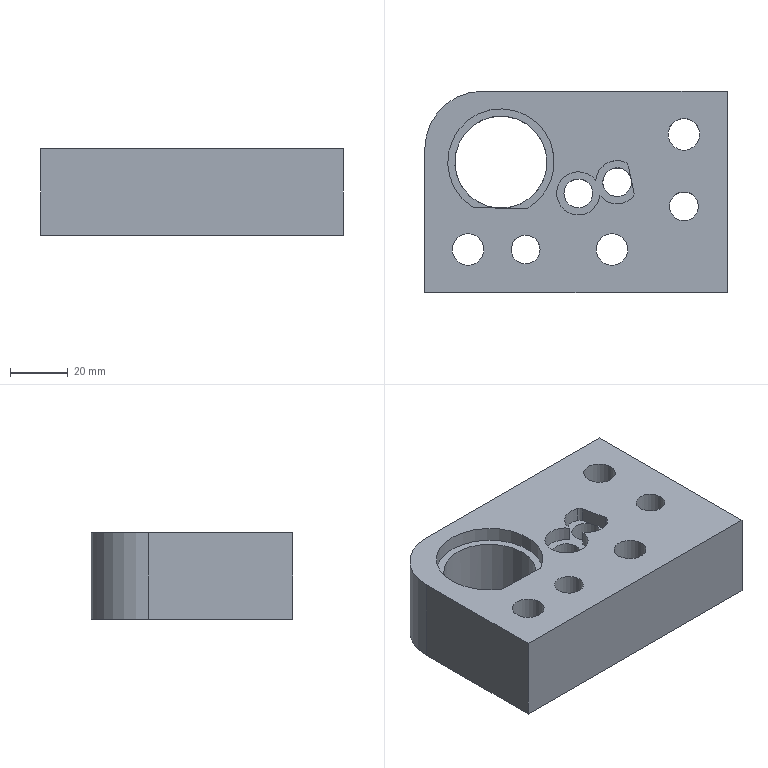Part | NX | features solid 2 | 1 solid | 33 faces | box 105 x 70 x 30 mm | volume 169797 mm3 | cylinder 20 | plane 13 | commonest cylinder face diameters 4 x4 10 x4 11 x3 15 x3 17 x3 32 x1
STEP:
#1=CARTESIAN_POINT('',(-270.,215.,109.));
#2=VERTEX_POINT('',#1);
#3=CARTESIAN_POINT('',(-275.,215.,109.));
#4=DIRECTION('',(0.,0.,1.));
#5=DIRECTION('',(1.,0.,0.));
#6=AXIS2_PLACEMENT_3D('',#3,#4,#5);
#7=CIRCLE('',#6,5.);
#8=EDGE_CURVE('',#2,#2,#7,.T.);
#9=ORIENTED_EDGE('',*,*,#8,.F.);
#10=EDGE_LOOP('',(#9));
#11=FACE_BOUND('',#10,.T.);
#12=CARTESIAN_POINT('',(-215.,230.,109.));
#13=VERTEX_POINT('',#12);
#14=CARTESIAN_POINT('',(-220.,230.,109.));
#15=DIRECTION('',(0.,0.,1.));
#16=DIRECTION('',(1.,0.,0.));
#17=AXIS2_PLACEMENT_3D('',#14,#15,#16);
#18=CIRCLE('',#17,5.);
#19=EDGE_CURVE('',#13,#13,#18,.T.);
#20=ORIENTED_EDGE('',*,*,#19,.F.);
#21=EDGE_LOOP('',(#20));
#22=FACE_BOUND('',#21,.T.);
#23=CARTESIAN_POINT('',(-289.5,215.,109.));
#24=VERTEX_POINT('',#23);
#25=CARTESIAN_POINT('',(-295.,215.,109.));
#26=DIRECTION('',(0.,0.,1.));
#27=DIRECTION('',(1.,0.,0.));
#28=AXIS2_PLACEMENT_3D('',#25,#26,#27);
#29=CIRCLE('',#28,5.5);
#30=EDGE_CURVE('',#24,#24,#29,.T.);
#31=ORIENTED_EDGE('',*,*,#30,.F.);
#32=EDGE_LOOP('',(#31));
#33=FACE_BOUND('',#32,.T.);
#34=CARTESIAN_POINT('',(-239.5,215.,109.));
#35=VERTEX_POINT('',#34);
#36=CARTESIAN_POINT('',(-245.,215.,109.));
#37=DIRECTION('',(0.,0.,1.));
#38=DIRECTION('',(1.,0.,0.));
#39=AXIS2_PLACEMENT_3D('',#36,#37,#38);
#40=CIRCLE('',#39,5.5);
#41=EDGE_CURVE('',#35,#35,#40,.T.);
#42=ORIENTED_EDGE('',*,*,#41,.F.);
#43=EDGE_LOOP('',(#42));
#44=FACE_BOUND('',#43,.T.);
#45=CARTESIAN_POINT('',(-214.5,255.,109.));
#46=VERTEX_POINT('',#45);
#47=CARTESIAN_POINT('',(-220.,255.,109.));
#48=DIRECTION('',(0.,0.,1.));
#49=DIRECTION('',(1.,0.,0.));
#50=AXIS2_PLACEMENT_3D('',#47,#48,#49);
#51=CIRCLE('',#50,5.5);
#52=EDGE_CURVE('',#46,#46,#51,.T.);
#53=ORIENTED_EDGE('',*,*,#52,.F.);
#54=EDGE_LOOP('',(#53));
#55=FACE_BOUND('',#54,.T.);
#56=CARTESIAN_POINT('',(-292.747,229.61,109.));
#57=VERTEX_POINT('',#56);
#58=CARTESIAN_POINT('',(-275.289,229.126,109.));
#59=VERTEX_POINT('',#58);
#60=CARTESIAN_POINT('',(-201.051,227.07,109.));
#61=DIRECTION('',(0.9996,-0.0277,0.));
#62=VECTOR('',#61,1000.);
#63=LINE('',#60,#62);
#64=EDGE_CURVE('',#57,#59,#63,.T.);
#65=ORIENTED_EDGE('',*,*,#64,.F.);
#66=CARTESIAN_POINT('',(-293.797,229.942,109.));
#67=VERTEX_POINT('',#66);
#68=CARTESIAN_POINT('',(-292.692,231.609,109.));
#69=DIRECTION('',(0.,0.,1.));
#70=DIRECTION('',(1.,0.,0.));
#71=AXIS2_PLACEMENT_3D('',#68,#69,#70);
#72=CIRCLE('',#71,2.);
#73=EDGE_CURVE('',#57,#67,#72,.F.);
#74=ORIENTED_EDGE('',*,*,#73,.T.);
#75=CARTESIAN_POINT('',(-274.223,229.4,109.));
#76=VERTEX_POINT('',#75);
#77=CARTESIAN_POINT('',(-283.575,245.362,109.));
#78=DIRECTION('',(0.,0.,1.));
#79=DIRECTION('',(1.,0.,0.));
#80=AXIS2_PLACEMENT_3D('',#77,#78,#79);
#81=CIRCLE('',#80,18.5);
#82=EDGE_CURVE('',#67,#76,#81,.F.);
#83=ORIENTED_EDGE('',*,*,#82,.T.);
#84=CARTESIAN_POINT('',(-275.234,231.126,109.));
#85=DIRECTION('',(0.,0.,1.));
#86=DIRECTION('',(1.,0.,0.));
#87=AXIS2_PLACEMENT_3D('',#84,#85,#86);
#88=CIRCLE('',#87,2.);
#89=EDGE_CURVE('',#76,#59,#88,.F.);
#90=ORIENTED_EDGE('',*,*,#89,.T.);
#91=EDGE_LOOP('',(#65,#74,#83,#90));
#92=FACE_BOUND('',#91,.T.);
#93=CARTESIAN_POINT('',(-290.,270.,109.));
#94=VERTEX_POINT('',#93);
#95=CARTESIAN_POINT('',(-205.,270.,109.));
#96=VERTEX_POINT('',#95);
#97=CARTESIAN_POINT('',(-310.,270.,109.));
#98=DIRECTION('',(1.,0.,0.));
#99=VECTOR('',#98,1000.);
#100=LINE('',#97,#99);
#101=EDGE_CURVE('',#94,#96,#100,.T.);
#102=ORIENTED_EDGE('',*,*,#101,.F.);
#103=CARTESIAN_POINT('',(-310.,250.,109.));
#104=VERTEX_POINT('',#103);
#105=CARTESIAN_POINT('',(-290.,250.,109.));
#106=DIRECTION('',(0.,0.,1.));
#107=DIRECTION('',(1.,0.,0.));
#108=AXIS2_PLACEMENT_3D('',#105,#106,#107);
#109=CIRCLE('',#108,20.);
#110=EDGE_CURVE('',#94,#104,#109,.T.);
#111=ORIENTED_EDGE('',*,*,#110,.T.);
#112=CARTESIAN_POINT('',(-310.,200.,109.));
#113=VERTEX_POINT('',#112);
#114=CARTESIAN_POINT('',(-310.,200.,109.));
#115=DIRECTION('',(0.,1.,0.));
#116=VECTOR('',#115,1000.);
#117=LINE('',#114,#116);
#118=EDGE_CURVE('',#113,#104,#117,.T.);
#119=ORIENTED_EDGE('',*,*,#118,.F.);
#120=CARTESIAN_POINT('',(-205.,200.,109.));
#121=VERTEX_POINT('',#120);
#122=CARTESIAN_POINT('',(-310.,200.,109.));
#123=DIRECTION('',(1.,0.,0.));
#124=VECTOR('',#123,1000.);
#125=LINE('',#122,#124);
#126=EDGE_CURVE('',#113,#121,#125,.T.);
#127=ORIENTED_EDGE('',*,*,#126,.T.);
#128=CARTESIAN_POINT('',(-205.,200.,109.));
#129=DIRECTION('',(0.,1.,0.));
#130=VECTOR('',#129,1000.);
#131=LINE('',#128,#130);
#132=EDGE_CURVE('',#121,#96,#131,.T.);
#133=ORIENTED_EDGE('',*,*,#132,.T.);
#134=EDGE_LOOP('',(#102,#111,#119,#127,#133));
#135=FACE_BOUND('',#134,.T.);
#136=CARTESIAN_POINT('',(-237.37,234.9,109.));
#137=VERTEX_POINT('',#136);
#138=CARTESIAN_POINT('',(-239.275,243.92,109.));
#139=VERTEX_POINT('',#138);
#140=CARTESIAN_POINT('',(-241.86,256.158,109.));
#141=DIRECTION('',(-0.2067,0.9784,0.));
#142=VECTOR('',#141,1000.);
#143=LINE('',#140,#142);
#144=EDGE_CURVE('',#137,#139,#143,.T.);
#145=ORIENTED_EDGE('',*,*,#144,.F.);
#146=CARTESIAN_POINT('',(-237.913,233.072,109.));
#147=VERTEX_POINT('',#146);
#148=CARTESIAN_POINT('',(-239.326,234.486,109.));
#149=DIRECTION('',(0.,0.,1.));
#150=DIRECTION('',(1.,0.,0.));
#151=AXIS2_PLACEMENT_3D('',#148,#149,#150);
#152=CIRCLE('',#151,2.);
#153=EDGE_CURVE('',#137,#147,#152,.F.);
#154=ORIENTED_EDGE('',*,*,#153,.T.);
#155=CARTESIAN_POINT('',(-249.23,233.898,109.));
#156=VERTEX_POINT('',#155);
#157=CARTESIAN_POINT('',(-243.214,238.377,109.));
#158=DIRECTION('',(0.,0.,1.));
#159=DIRECTION('',(1.,0.,0.));
#160=AXIS2_PLACEMENT_3D('',#157,#158,#159);
#161=CIRCLE('',#160,7.5);
#162=EDGE_CURVE('',#147,#156,#161,.F.);
#163=ORIENTED_EDGE('',*,*,#162,.T.);
#164=CARTESIAN_POINT('',(-250.689,238.992,109.));
#165=VERTEX_POINT('',#164);
#166=CARTESIAN_POINT('',(-256.705,234.513,109.));
#167=DIRECTION('',(0.,0.,1.));
#168=DIRECTION('',(1.,0.,0.));
#169=AXIS2_PLACEMENT_3D('',#166,#167,#168);
#170=CIRCLE('',#169,7.5);
#171=EDGE_CURVE('',#156,#165,#170,.F.);
#172=ORIENTED_EDGE('',*,*,#171,.T.);
#173=CARTESIAN_POINT('',(-240.511,245.373,109.));
#174=VERTEX_POINT('',#173);
#175=CARTESIAN_POINT('',(-243.214,238.377,109.));
#176=DIRECTION('',(0.,0.,1.));
#177=DIRECTION('',(1.,0.,0.));
#178=AXIS2_PLACEMENT_3D('',#175,#176,#177);
#179=CIRCLE('',#178,7.5);
#180=EDGE_CURVE('',#165,#174,#179,.F.);
#181=ORIENTED_EDGE('',*,*,#180,.T.);
#182=CARTESIAN_POINT('',(-241.232,243.507,109.));
#183=DIRECTION('',(0.,0.,1.));
#184=DIRECTION('',(1.,0.,0.));
#185=AXIS2_PLACEMENT_3D('',#182,#183,#184);
#186=CIRCLE('',#185,2.);
#187=EDGE_CURVE('',#174,#139,#186,.F.);
#188=ORIENTED_EDGE('',*,*,#187,.T.);
#189=EDGE_LOOP('',(#145,#154,#163,#172,#181,#188));
#190=FACE_BOUND('',#189,.T.);
#191=CARTESIAN_POINT('',(-200.,265.,109.));
#192=DIRECTION('',(0.,0.,1.));
#193=DIRECTION('',(1.,0.,0.));
#194=AXIS2_PLACEMENT_3D('',#191,#192,#193);
#195=PLANE('',#194);
#196=ADVANCED_FACE('',(#11,#22,#33,#44,#55,#92,#135,#190),#195,.T.);
#197=CARTESIAN_POINT('',(-238.214,238.377,79.));
#198=VERTEX_POINT('',#197);
#199=CARTESIAN_POINT('',(-243.214,238.377,79.));
#200=DIRECTION('',(0.,0.,1.));
#201=DIRECTION('',(1.,0.,0.));
#202=AXIS2_PLACEMENT_3D('',#199,#200,#201);
#203=CIRCLE('',#202,5.);
#204=EDGE_CURVE('',#198,#198,#203,.T.);
#205=ORIENTED_EDGE('',*,*,#204,.F.);
#206=EDGE_LOOP('',(#205));
#207=FACE_BOUND('',#206,.T.);
#208=CARTESIAN_POINT('',(-238.322,239.41,104.));
#209=VERTEX_POINT('',#208);
#210=CARTESIAN_POINT('',(-243.214,238.377,104.));
#211=DIRECTION('',(0.,0.,1.));
#212=DIRECTION('',(1.,0.,0.));
#213=AXIS2_PLACEMENT_3D('',#210,#211,#212);
#214=CIRCLE('',#213,5.);
#215=EDGE_CURVE('',#209,#209,#214,.F.);
#216=ORIENTED_EDGE('',*,*,#215,.F.);
#217=EDGE_LOOP('',(#216));
#218=FACE_BOUND('',#217,.T.);
#219=CARTESIAN_POINT('',(-243.214,238.377,-452.));
#220=DIRECTION('',(0.,0.,1.));
#221=DIRECTION('',(1.,0.,0.));
#222=AXIS2_PLACEMENT_3D('',#219,#220,#221);
#223=CYLINDRICAL_SURFACE('',#222,5.);
#224=ADVANCED_FACE('',(#207,#218),#223,.F.);
#225=ORIENTED_EDGE('',*,*,#171,.F.);
#226=CARTESIAN_POINT('',(-249.23,233.898,104.));
#227=VERTEX_POINT('',#226);
#228=CARTESIAN_POINT('',(-249.23,233.898,111.5));
#229=DIRECTION('',(0.,0.,-1.));
#230=VECTOR('',#229,1000.);
#231=LINE('',#228,#230);
#232=EDGE_CURVE('',#156,#227,#231,.T.);
#233=ORIENTED_EDGE('',*,*,#232,.T.);
#234=CARTESIAN_POINT('',(-250.689,238.992,104.));
#235=VERTEX_POINT('',#234);
#236=CARTESIAN_POINT('',(-256.705,234.513,104.));
#237=DIRECTION('',(0.,0.,1.));
#238=DIRECTION('',(1.,0.,0.));
#239=AXIS2_PLACEMENT_3D('',#236,#237,#238);
#240=CIRCLE('',#239,7.5);
#241=EDGE_CURVE('',#235,#227,#240,.T.);
#242=ORIENTED_EDGE('',*,*,#241,.F.);
#243=CARTESIAN_POINT('',(-250.689,238.992,111.5));
#244=DIRECTION('',(0.,0.,-1.));
#245=VECTOR('',#244,1000.);
#246=LINE('',#243,#245);
#247=EDGE_CURVE('',#235,#165,#246,.F.);
#248=ORIENTED_EDGE('',*,*,#247,.T.);
#249=EDGE_LOOP('',(#225,#233,#242,#248));
#250=FACE_BOUND('',#249,.T.);
#251=CARTESIAN_POINT('',(-256.705,234.513,119.));
#252=DIRECTION('',(0.,0.,-1.));
#253=DIRECTION('',(-1.,0.,0.));
#254=AXIS2_PLACEMENT_3D('',#251,#252,#253);
#255=CYLINDRICAL_SURFACE('',#254,7.5);
#256=ADVANCED_FACE('',(#250),#255,.F.);
#257=CARTESIAN_POINT('',(-251.705,234.513,79.));
#258=VERTEX_POINT('',#257);
#259=CARTESIAN_POINT('',(-256.705,234.513,79.));
#260=DIRECTION('',(0.,0.,1.));
#261=DIRECTION('',(1.,0.,0.));
#262=AXIS2_PLACEMENT_3D('',#259,#260,#261);
#263=CIRCLE('',#262,5.);
#264=EDGE_CURVE('',#258,#258,#263,.T.);
#265=ORIENTED_EDGE('',*,*,#264,.F.);
#266=EDGE_LOOP('',(#265));
#267=FACE_BOUND('',#266,.T.);
#268=CARTESIAN_POINT('',(-251.705,234.513,104.));
#269=VERTEX_POINT('',#268);
#270=CARTESIAN_POINT('',(-256.705,234.513,104.));
#271=DIRECTION('',(0.,0.,1.));
#272=DIRECTION('',(1.,0.,0.));
#273=AXIS2_PLACEMENT_3D('',#270,#271,#272);
#274=CIRCLE('',#273,5.);
#275=EDGE_CURVE('',#269,#269,#274,.F.);
#276=ORIENTED_EDGE('',*,*,#275,.F.);
#277=EDGE_LOOP('',(#276));
#278=FACE_BOUND('',#277,.T.);
#279=CARTESIAN_POINT('',(-256.705,234.513,-452.));
#280=DIRECTION('',(0.,0.,1.));
#281=DIRECTION('',(1.,0.,0.));
#282=AXIS2_PLACEMENT_3D('',#279,#280,#281);
#283=CYLINDRICAL_SURFACE('',#282,5.);
#284=ADVANCED_FACE('',(#267,#278),#283,.F.);
#285=CARTESIAN_POINT('',(-267.575,245.362,79.));
#286=VERTEX_POINT('',#285);
#287=CARTESIAN_POINT('',(-283.575,245.362,79.));
#288=DIRECTION('',(0.,0.,1.));
#289=DIRECTION('',(1.,0.,0.));
#290=AXIS2_PLACEMENT_3D('',#287,#288,#289);
#291=CIRCLE('',#290,16.);
#292=EDGE_CURVE('',#286,#286,#291,.T.);
#293=ORIENTED_EDGE('',*,*,#292,.F.);
#294=EDGE_LOOP('',(#293));
#295=FACE_BOUND('',#294,.T.);
#296=CARTESIAN_POINT('',(-284.018,229.368,104.));
#297=VERTEX_POINT('',#296);
#298=CARTESIAN_POINT('',(-283.575,245.362,104.));
#299=DIRECTION('',(0.,0.,1.));
#300=DIRECTION('',(1.,0.,0.));
#301=AXIS2_PLACEMENT_3D('',#298,#299,#300);
#302=CIRCLE('',#301,16.);
#303=EDGE_CURVE('',#297,#297,#302,.F.);
#304=ORIENTED_EDGE('',*,*,#303,.F.);
#305=EDGE_LOOP('',(#304));
#306=FACE_BOUND('',#305,.T.);
#307=CARTESIAN_POINT('',(-283.575,245.362,-446.));
#308=DIRECTION('',(0.,0.,1.));
#309=DIRECTION('',(1.,0.,0.));
#310=AXIS2_PLACEMENT_3D('',#307,#308,#309);
#311=CYLINDRICAL_SURFACE('',#310,16.);
#312=ADVANCED_FACE('',(#295,#306),#311,.F.);
#313=CARTESIAN_POINT('',(-290.,270.,79.));
#314=VERTEX_POINT('',#313);
#315=CARTESIAN_POINT('',(-205.,270.,79.));
#316=VERTEX_POINT('',#315);
#317=CARTESIAN_POINT('',(-310.,270.,79.));
#318=DIRECTION('',(1.,0.,0.));
#319=VECTOR('',#318,1000.);
#320=LINE('',#317,#319);
#321=EDGE_CURVE('',#314,#316,#320,.T.);
#322=ORIENTED_EDGE('',*,*,#321,.F.);
#323=CARTESIAN_POINT('',(-290.,270.,109.));
#324=DIRECTION('',(0.,0.,-1.));
#325=VECTOR('',#324,1000.);
#326=LINE('',#323,#325);
#327=EDGE_CURVE('',#314,#94,#326,.F.);
#328=ORIENTED_EDGE('',*,*,#327,.T.);
#329=ORIENTED_EDGE('',*,*,#101,.T.);
#330=CARTESIAN_POINT('',(-205.,270.,109.));
#331=DIRECTION('',(0.,0.,-1.));
#332=VECTOR('',#331,1000.);
#333=LINE('',#330,#332);
#334=EDGE_CURVE('',#96,#316,#333,.T.);
#335=ORIENTED_EDGE('',*,*,#334,.T.);
#336=EDGE_LOOP('',(#322,#328,#329,#335));
#337=FACE_BOUND('',#336,.T.);
#338=CARTESIAN_POINT('',(-310.,270.,109.));
#339=DIRECTION('',(0.,1.,0.));
#340=DIRECTION('',(0.,0.,1.));
#341=AXIS2_PLACEMENT_3D('',#338,#339,#340);
#342=PLANE('',#341);
#343=ADVANCED_FACE('',(#337),#342,.T.);
#344=CARTESIAN_POINT('',(-205.,200.,79.));
#345=VERTEX_POINT('',#344);
#346=CARTESIAN_POINT('',(-205.,200.,79.));
#347=DIRECTION('',(0.,1.,0.));
#348=VECTOR('',#347,1000.);
#349=LINE('',#346,#348);
#350=EDGE_CURVE('',#345,#316,#349,.T.);
#351=ORIENTED_EDGE('',*,*,#350,.T.);
#352=ORIENTED_EDGE('',*,*,#334,.F.);
#353=ORIENTED_EDGE('',*,*,#132,.F.);
#354=CARTESIAN_POINT('',(-205.,200.,109.));
#355=DIRECTION('',(0.,0.,-1.));
#356=VECTOR('',#355,1000.);
#357=LINE('',#354,#356);
#358=EDGE_CURVE('',#121,#345,#357,.T.);
#359=ORIENTED_EDGE('',*,*,#358,.T.);
#360=EDGE_LOOP('',(#351,#352,#353,#359));
#361=FACE_BOUND('',#360,.T.);
#362=CARTESIAN_POINT('',(-205.,200.,109.));
#363=DIRECTION('',(-1.,0.,0.));
#364=DIRECTION('',(0.,0.,1.));
#365=AXIS2_PLACEMENT_3D('',#362,#363,#364);
#366=PLANE('',#365);
#367=ADVANCED_FACE('',(#361),#366,.F.);
#368=CARTESIAN_POINT('',(-310.,200.,79.));
#369=VERTEX_POINT('',#368);
#370=CARTESIAN_POINT('',(-310.,200.,79.));
#371=DIRECTION('',(1.,0.,0.));
#372=VECTOR('',#371,1000.);
#373=LINE('',#370,#372);
#374=EDGE_CURVE('',#369,#345,#373,.T.);
#375=ORIENTED_EDGE('',*,*,#374,.T.);
#376=ORIENTED_EDGE('',*,*,#358,.F.);
#377=ORIENTED_EDGE('',*,*,#126,.F.);
#378=CARTESIAN_POINT('',(-310.,200.,109.));
#379=DIRECTION('',(0.,0.,-1.));
#380=VECTOR('',#379,1000.);
#381=LINE('',#378,#380);
#382=EDGE_CURVE('',#113,#369,#381,.T.);
#383=ORIENTED_EDGE('',*,*,#382,.T.);
#384=EDGE_LOOP('',(#375,#376,#377,#383));
#385=FACE_BOUND('',#384,.T.);
#386=CARTESIAN_POINT('',(-310.,200.,109.));
#387=DIRECTION('',(0.,1.,0.));
#388=DIRECTION('',(0.,0.,1.));
#389=AXIS2_PLACEMENT_3D('',#386,#387,#388);
#390=PLANE('',#389);
#391=ADVANCED_FACE('',(#385),#390,.F.);
#392=ORIENTED_EDGE('',*,*,#118,.T.);
#393=CARTESIAN_POINT('',(-310.,250.,79.));
#394=VERTEX_POINT('',#393);
#395=CARTESIAN_POINT('',(-310.,250.,109.));
#396=DIRECTION('',(0.,0.,-1.));
#397=VECTOR('',#396,1000.);
#398=LINE('',#395,#397);
#399=EDGE_CURVE('',#104,#394,#398,.T.);
#400=ORIENTED_EDGE('',*,*,#399,.T.);
#401=CARTESIAN_POINT('',(-310.,200.,79.));
#402=DIRECTION('',(0.,1.,0.));
#403=VECTOR('',#402,1000.);
#404=LINE('',#401,#403);
#405=EDGE_CURVE('',#369,#394,#404,.T.);
#406=ORIENTED_EDGE('',*,*,#405,.F.);
#407=ORIENTED_EDGE('',*,*,#382,.F.);
#408=EDGE_LOOP('',(#392,#400,#406,#407));
#409=FACE_BOUND('',#408,.T.);
#410=CARTESIAN_POINT('',(-310.,200.,109.));
#411=DIRECTION('',(-1.,0.,0.));
#412=DIRECTION('',(0.,0.,1.));
#413=AXIS2_PLACEMENT_3D('',#410,#411,#412);
#414=PLANE('',#413);
#415=ADVANCED_FACE('',(#409),#414,.T.);
#416=CARTESIAN_POINT('',(-270.,215.,79.));
#417=VERTEX_POINT('',#416);
#418=CARTESIAN_POINT('',(-275.,215.,79.));
#419=DIRECTION('',(0.,0.,1.));
#420=DIRECTION('',(1.,0.,0.));
#421=AXIS2_PLACEMENT_3D('',#418,#419,#420);
#422=CIRCLE('',#421,5.);
#423=EDGE_CURVE('',#417,#417,#422,.T.);
#424=ORIENTED_EDGE('',*,*,#423,.T.);
#425=EDGE_LOOP('',(#424));
#426=FACE_BOUND('',#425,.T.);
#427=CARTESIAN_POINT('',(-215.,230.,79.));
#428=VERTEX_POINT('',#427);
#429=CARTESIAN_POINT('',(-220.,230.,79.));
#430=DIRECTION('',(0.,0.,1.));
#431=DIRECTION('',(1.,0.,0.));
#432=AXIS2_PLACEMENT_3D('',#429,#430,#431);
#433=CIRCLE('',#432,5.);
#434=EDGE_CURVE('',#428,#428,#433,.T.);
#435=ORIENTED_EDGE('',*,*,#434,.T.);
#436=EDGE_LOOP('',(#435));
#437=FACE_BOUND('',#436,.T.);
#438=CARTESIAN_POINT('',(-286.5,215.,79.));
#439=VERTEX_POINT('',#438);
#440=CARTESIAN_POINT('',(-295.,215.,79.));
#441=DIRECTION('',(0.,0.,1.));
#442=DIRECTION('',(1.,0.,0.));
#443=AXIS2_PLACEMENT_3D('',#440,#441,#442);
#444=CIRCLE('',#443,8.5);
#445=EDGE_CURVE('',#439,#439,#444,.T.);
#446=ORIENTED_EDGE('',*,*,#445,.T.);
#447=EDGE_LOOP('',(#446));
#448=FACE_BOUND('',#447,.T.);
#449=CARTESIAN_POINT('',(-236.5,215.,79.));
#450=VERTEX_POINT('',#449);
#451=CARTESIAN_POINT('',(-245.,215.,79.));
#452=DIRECTION('',(0.,0.,1.));
#453=DIRECTION('',(1.,0.,0.));
#454=AXIS2_PLACEMENT_3D('',#451,#452,#453);
#455=CIRCLE('',#454,8.5);
#456=EDGE_CURVE('',#450,#450,#455,.T.);
#457=ORIENTED_EDGE('',*,*,#456,.T.);
#458=EDGE_LOOP('',(#457));
#459=FACE_BOUND('',#458,.T.);
#460=CARTESIAN_POINT('',(-211.5,255.,79.));
#461=VERTEX_POINT('',#460);
#462=CARTESIAN_POINT('',(-220.,255.,79.));
#463=DIRECTION('',(0.,0.,1.));
#464=DIRECTION('',(1.,0.,0.));
#465=AXIS2_PLACEMENT_3D('',#462,#463,#464);
#466=CIRCLE('',#465,8.5);
#467=EDGE_CURVE('',#461,#461,#466,.T.);
#468=ORIENTED_EDGE('',*,*,#467,.T.);
#469=EDGE_LOOP('',(#468));
#470=FACE_BOUND('',#469,.T.);
#471=ORIENTED_EDGE('',*,*,#204,.T.);
#472=EDGE_LOOP('',(#471));
#473=FACE_BOUND('',#472,.T.);
#474=ORIENTED_EDGE('',*,*,#264,.T.);
#475=EDGE_LOOP('',(#474));
#476=FACE_BOUND('',#475,.T.);
#477=ORIENTED_EDGE('',*,*,#292,.T.);
#478=EDGE_LOOP('',(#477));
#479=FACE_BOUND('',#478,.T.);
#480=ORIENTED_EDGE('',*,*,#405,.T.);
#481=CARTESIAN_POINT('',(-290.,250.,79.));
#482=DIRECTION('',(0.,0.,1.));
#483=DIRECTION('',(1.,0.,0.));
#484=AXIS2_PLACEMENT_3D('',#481,#482,#483);
#485=CIRCLE('',#484,20.);
#486=EDGE_CURVE('',#394,#314,#485,.F.);
#487=ORIENTED_EDGE('',*,*,#486,.T.);
#488=ORIENTED_EDGE('',*,*,#321,.T.);
#489=ORIENTED_EDGE('',*,*,#350,.F.);
#490=ORIENTED_EDGE('',*,*,#374,.F.);
#491=EDGE_LOOP('',(#480,#487,#488,#489,#490));
#492=FACE_BOUND('',#491,.T.);
#493=CARTESIAN_POINT('',(-200.,265.,79.));
#494=DIRECTION('',(0.,0.,1.));
#495=DIRECTION('',(1.,0.,0.));
#496=AXIS2_PLACEMENT_3D('',#493,#494,#495);
#497=PLANE('',#496);
#498=ADVANCED_FACE('',(#426,#437,#448,#459,#470,#473,#476,#479,#492),#497,.F.);
#499=CARTESIAN_POINT('',(-292.747,229.61,104.));
#500=VERTEX_POINT('',#499);
#501=CARTESIAN_POINT('',(-284.018,229.368,104.));
#502=DIRECTION('',(-0.9996,0.0277,0.));
#503=VECTOR('',#502,1000.);
#504=LINE('',#501,#503);
#505=EDGE_CURVE('',#297,#500,#504,.T.);
#506=ORIENTED_EDGE('',*,*,#505,.T.);
#507=CARTESIAN_POINT('',(-292.747,229.61,119.));
#508=DIRECTION('',(0.,0.,-1.));
#509=VECTOR('',#508,1000.);
#510=LINE('',#507,#509);
#511=EDGE_CURVE('',#500,#57,#510,.F.);
#512=ORIENTED_EDGE('',*,*,#511,.T.);
#513=ORIENTED_EDGE('',*,*,#64,.T.);
#514=CARTESIAN_POINT('',(-275.289,229.126,104.));
#515=VERTEX_POINT('',#514);
#516=CARTESIAN_POINT('',(-275.289,229.126,119.));
#517=DIRECTION('',(0.,0.,-1.));
#518=VECTOR('',#517,1000.);
#519=LINE('',#516,#518);
#520=EDGE_CURVE('',#59,#515,#519,.T.);
#521=ORIENTED_EDGE('',*,*,#520,.T.);
#522=CARTESIAN_POINT('',(-284.018,229.368,104.));
#523=DIRECTION('',(-0.9996,0.0277,0.));
#524=VECTOR('',#523,1000.);
#525=LINE('',#522,#524);
#526=EDGE_CURVE('',#515,#297,#525,.T.);
#527=ORIENTED_EDGE('',*,*,#526,.T.);
#528=EDGE_LOOP('',(#506,#512,#513,#521,#527));
#529=FACE_BOUND('',#528,.T.);
#530=CARTESIAN_POINT('',(-284.018,229.368,119.));
#531=DIRECTION('',(-0.0277,-0.9996,0.));
#532=DIRECTION('',(0.9996,-0.0277,0.));
#533=AXIS2_PLACEMENT_3D('',#530,#531,#532);
#534=PLANE('',#533);
#535=ADVANCED_FACE('',(#529),#534,.F.);
#536=CARTESIAN_POINT('',(-274.223,229.4,104.));
#537=VERTEX_POINT('',#536);
#538=CARTESIAN_POINT('',(-293.797,229.942,104.));
#539=VERTEX_POINT('',#538);
#540=CARTESIAN_POINT('',(-283.575,245.362,104.));
#541=DIRECTION('',(0.,0.,1.));
#542=DIRECTION('',(1.,0.,0.));
#543=AXIS2_PLACEMENT_3D('',#540,#541,#542);
#544=CIRCLE('',#543,18.5);
#545=EDGE_CURVE('',#537,#539,#544,.T.);
#546=ORIENTED_EDGE('',*,*,#545,.T.);
#547=CARTESIAN_POINT('',(-292.692,231.609,104.));
#548=DIRECTION('',(0.,0.,1.));
#549=DIRECTION('',(1.,0.,0.));
#550=AXIS2_PLACEMENT_3D('',#547,#548,#549);
#551=CIRCLE('',#550,2.);
#552=EDGE_CURVE('',#539,#500,#551,.T.);
#553=ORIENTED_EDGE('',*,*,#552,.T.);
#554=ORIENTED_EDGE('',*,*,#505,.F.);
#555=ORIENTED_EDGE('',*,*,#303,.T.);
#556=ORIENTED_EDGE('',*,*,#526,.F.);
#557=CARTESIAN_POINT('',(-275.234,231.126,104.));
#558=DIRECTION('',(0.,0.,1.));
#559=DIRECTION('',(1.,0.,0.));
#560=AXIS2_PLACEMENT_3D('',#557,#558,#559);
#561=CIRCLE('',#560,2.);
#562=EDGE_CURVE('',#515,#537,#561,.T.);
#563=ORIENTED_EDGE('',*,*,#562,.T.);
#564=EDGE_LOOP('',(#546,#553,#554,#555,#556,#563));
#565=FACE_BOUND('',#564,.T.);
#566=CARTESIAN_POINT('',(-283.575,245.362,104.));
#567=DIRECTION('',(0.,0.,1.));
#568=DIRECTION('',(0.0277,0.9996,0.));
#569=AXIS2_PLACEMENT_3D('',#566,#567,#568);
#570=PLANE('',#569);
#571=ADVANCED_FACE('',(#565),#570,.T.);
#572=ORIENTED_EDGE('',*,*,#82,.F.);
#573=CARTESIAN_POINT('',(-293.797,229.942,119.));
#574=DIRECTION('',(0.,0.,-1.));
#575=VECTOR('',#574,1000.);
#576=LINE('',#573,#575);
#577=EDGE_CURVE('',#67,#539,#576,.T.);
#578=ORIENTED_EDGE('',*,*,#577,.T.);
#579=ORIENTED_EDGE('',*,*,#545,.F.);
#580=CARTESIAN_POINT('',(-274.223,229.4,119.));
#581=DIRECTION('',(0.,0.,-1.));
#582=VECTOR('',#581,1000.);
#583=LINE('',#580,#582);
#584=EDGE_CURVE('',#537,#76,#583,.F.);
#585=ORIENTED_EDGE('',*,*,#584,.T.);
#586=EDGE_LOOP('',(#572,#578,#579,#585));
#587=FACE_BOUND('',#586,.T.);
#588=CARTESIAN_POINT('',(-283.575,245.362,119.));
#589=DIRECTION('',(0.,0.,-1.));
#590=DIRECTION('',(-1.,0.,0.));
#591=AXIS2_PLACEMENT_3D('',#588,#589,#590);
#592=CYLINDRICAL_SURFACE('',#591,18.5);
#593=ADVANCED_FACE('',(#587),#592,.F.);
#594=CARTESIAN_POINT('',(-239.275,243.92,104.));
#595=VERTEX_POINT('',#594);
#596=CARTESIAN_POINT('',(-238.322,239.41,104.));
#597=DIRECTION('',(0.2067,-0.9784,0.));
#598=VECTOR('',#597,1000.);
#599=LINE('',#596,#598);
#600=EDGE_CURVE('',#595,#209,#599,.T.);
#601=ORIENTED_EDGE('',*,*,#600,.F.);
#602=CARTESIAN_POINT('',(-240.511,245.373,104.));
#603=VERTEX_POINT('',#602);
#604=CARTESIAN_POINT('',(-241.232,243.507,104.));
#605=DIRECTION('',(0.,0.,1.));
#606=DIRECTION('',(1.,0.,0.));
#607=AXIS2_PLACEMENT_3D('',#604,#605,#606);
#608=CIRCLE('',#607,2.);
#609=EDGE_CURVE('',#595,#603,#608,.T.);
#610=ORIENTED_EDGE('',*,*,#609,.T.);
#611=CARTESIAN_POINT('',(-243.214,238.377,104.));
#612=DIRECTION('',(0.,0.,1.));
#613=DIRECTION('',(1.,0.,0.));
#614=AXIS2_PLACEMENT_3D('',#611,#612,#613);
#615=CIRCLE('',#614,7.5);
#616=EDGE_CURVE('',#603,#235,#615,.T.);
#617=ORIENTED_EDGE('',*,*,#616,.T.);
#618=ORIENTED_EDGE('',*,*,#241,.T.);
#619=CARTESIAN_POINT('',(-237.913,233.072,104.));
#620=VERTEX_POINT('',#619);
#621=CARTESIAN_POINT('',(-243.214,238.377,104.));
#622=DIRECTION('',(0.,0.,1.));
#623=DIRECTION('',(1.,0.,0.));
#624=AXIS2_PLACEMENT_3D('',#621,#622,#623);
#625=CIRCLE('',#624,7.5);
#626=EDGE_CURVE('',#227,#620,#625,.T.);
#627=ORIENTED_EDGE('',*,*,#626,.T.);
#628=CARTESIAN_POINT('',(-237.37,234.9,104.));
#629=VERTEX_POINT('',#628);
#630=CARTESIAN_POINT('',(-239.326,234.486,104.));
#631=DIRECTION('',(0.,0.,1.));
#632=DIRECTION('',(1.,0.,0.));
#633=AXIS2_PLACEMENT_3D('',#630,#631,#632);
#634=CIRCLE('',#633,2.);
#635=EDGE_CURVE('',#620,#629,#634,.T.);
#636=ORIENTED_EDGE('',*,*,#635,.T.);
#637=CARTESIAN_POINT('',(-238.322,239.41,104.));
#638=DIRECTION('',(0.2067,-0.9784,0.));
#639=VECTOR('',#638,1000.);
#640=LINE('',#637,#639);
#641=EDGE_CURVE('',#209,#629,#640,.T.);
#642=ORIENTED_EDGE('',*,*,#641,.F.);
#643=ORIENTED_EDGE('',*,*,#215,.T.);
#644=EDGE_LOOP('',(#601,#610,#617,#618,#627,#636,#642,#643));
#645=FACE_BOUND('',#644,.T.);
#646=ORIENTED_EDGE('',*,*,#275,.T.);
#647=EDGE_LOOP('',(#646));
#648=FACE_BOUND('',#647,.T.);
#649=CARTESIAN_POINT('',(-256.705,234.513,104.));
#650=DIRECTION('',(0.,0.,1.));
#651=DIRECTION('',(1.,0.,0.));
#652=AXIS2_PLACEMENT_3D('',#649,#650,#651);
#653=PLANE('',#652);
#654=ADVANCED_FACE('',(#645,#648),#653,.T.);
#655=ORIENTED_EDGE('',*,*,#144,.T.);
#656=CARTESIAN_POINT('',(-239.275,243.92,119.));
#657=DIRECTION('',(0.,0.,-1.));
#658=VECTOR('',#657,1000.);
#659=LINE('',#656,#658);
#660=EDGE_CURVE('',#139,#595,#659,.T.);
#661=ORIENTED_EDGE('',*,*,#660,.T.);
#662=ORIENTED_EDGE('',*,*,#600,.T.);
#663=ORIENTED_EDGE('',*,*,#641,.T.);
#664=CARTESIAN_POINT('',(-237.37,234.9,119.));
#665=DIRECTION('',(0.,0.,-1.));
#666=VECTOR('',#665,1000.);
#667=LINE('',#664,#666);
#668=EDGE_CURVE('',#629,#137,#667,.F.);
#669=ORIENTED_EDGE('',*,*,#668,.T.);
#670=EDGE_LOOP('',(#655,#661,#662,#663,#669));
#671=FACE_BOUND('',#670,.T.);
#672=CARTESIAN_POINT('',(-238.322,239.41,119.));
#673=DIRECTION('',(0.9784,0.2067,0.));
#674=DIRECTION('',(-0.2067,0.9784,0.));
#675=AXIS2_PLACEMENT_3D('',#672,#673,#674);
#676=PLANE('',#675);
#677=ADVANCED_FACE('',(#671),#676,.F.);
#678=ORIENTED_EDGE('',*,*,#162,.F.);
#679=CARTESIAN_POINT('',(-237.913,233.072,119.));
#680=DIRECTION('',(0.,0.,-1.));
#681=VECTOR('',#680,1000.);
#682=LINE('',#679,#681);
#683=EDGE_CURVE('',#147,#620,#682,.T.);
#684=ORIENTED_EDGE('',*,*,#683,.T.);
#685=ORIENTED_EDGE('',*,*,#626,.F.);
#686=ORIENTED_EDGE('',*,*,#232,.F.);
#687=EDGE_LOOP('',(#678,#684,#685,#686));
#688=FACE_BOUND('',#687,.T.);
#689=CARTESIAN_POINT('',(-243.214,238.377,119.));
#690=DIRECTION('',(0.,0.,-1.));
#691=DIRECTION('',(-1.,0.,0.));
#692=AXIS2_PLACEMENT_3D('',#689,#690,#691);
#693=CYLINDRICAL_SURFACE('',#692,7.5);
#694=ADVANCED_FACE('',(#688),#693,.F.);
#695=ORIENTED_EDGE('',*,*,#616,.F.);
#696=CARTESIAN_POINT('',(-240.511,245.373,119.));
#697=DIRECTION('',(0.,0.,-1.));
#698=VECTOR('',#697,1000.);
#699=LINE('',#696,#698);
#700=EDGE_CURVE('',#603,#174,#699,.F.);
#701=ORIENTED_EDGE('',*,*,#700,.T.);
#702=ORIENTED_EDGE('',*,*,#180,.F.);
#703=ORIENTED_EDGE('',*,*,#247,.F.);
#704=EDGE_LOOP('',(#695,#701,#702,#703));
#705=FACE_BOUND('',#704,.T.);
#706=CARTESIAN_POINT('',(-243.214,238.377,119.));
#707=DIRECTION('',(0.,0.,-1.));
#708=DIRECTION('',(-1.,0.,0.));
#709=AXIS2_PLACEMENT_3D('',#706,#707,#708);
#710=CYLINDRICAL_SURFACE('',#709,7.5);
#711=ADVANCED_FACE('',(#705),#710,.F.);
#712=ORIENTED_EDGE('',*,*,#153,.F.);
#713=ORIENTED_EDGE('',*,*,#668,.F.);
#714=ORIENTED_EDGE('',*,*,#635,.F.);
#715=ORIENTED_EDGE('',*,*,#683,.F.);
#716=EDGE_LOOP('',(#712,#713,#714,#715));
#717=FACE_BOUND('',#716,.T.);
#718=CARTESIAN_POINT('',(-239.326,234.486,119.));
#719=DIRECTION('',(0.,0.,-1.));
#720=DIRECTION('',(-1.,0.,0.));
#721=AXIS2_PLACEMENT_3D('',#718,#719,#720);
#722=CYLINDRICAL_SURFACE('',#721,2.);
#723=ADVANCED_FACE('',(#717),#722,.F.);
#724=ORIENTED_EDGE('',*,*,#187,.F.);
#725=ORIENTED_EDGE('',*,*,#700,.F.);
#726=ORIENTED_EDGE('',*,*,#609,.F.);
#727=ORIENTED_EDGE('',*,*,#660,.F.);
#728=EDGE_LOOP('',(#724,#725,#726,#727));
#729=FACE_BOUND('',#728,.T.);
#730=CARTESIAN_POINT('',(-241.232,243.507,119.));
#731=DIRECTION('',(0.,0.,-1.));
#732=DIRECTION('',(-1.,0.,0.));
#733=AXIS2_PLACEMENT_3D('',#730,#731,#732);
#734=CYLINDRICAL_SURFACE('',#733,2.);
#735=ADVANCED_FACE('',(#729),#734,.F.);
#736=ORIENTED_EDGE('',*,*,#89,.F.);
#737=ORIENTED_EDGE('',*,*,#584,.F.);
#738=ORIENTED_EDGE('',*,*,#562,.F.);
#739=ORIENTED_EDGE('',*,*,#520,.F.);
#740=EDGE_LOOP('',(#736,#737,#738,#739));
#741=FACE_BOUND('',#740,.T.);
#742=CARTESIAN_POINT('',(-275.234,231.126,119.));
#743=DIRECTION('',(0.,0.,-1.));
#744=DIRECTION('',(-1.,0.,0.));
#745=AXIS2_PLACEMENT_3D('',#742,#743,#744);
#746=CYLINDRICAL_SURFACE('',#745,2.);
#747=ADVANCED_FACE('',(#741),#746,.F.);
#748=ORIENTED_EDGE('',*,*,#73,.F.);
#749=ORIENTED_EDGE('',*,*,#511,.F.);
#750=ORIENTED_EDGE('',*,*,#552,.F.);
#751=ORIENTED_EDGE('',*,*,#577,.F.);
#752=EDGE_LOOP('',(#748,#749,#750,#751));
#753=FACE_BOUND('',#752,.T.);
#754=CARTESIAN_POINT('',(-292.692,231.609,119.));
#755=DIRECTION('',(0.,0.,-1.));
#756=DIRECTION('',(-1.,0.,0.));
#757=AXIS2_PLACEMENT_3D('',#754,#755,#756);
#758=CYLINDRICAL_SURFACE('',#757,2.);
#759=ADVANCED_FACE('',(#753),#758,.F.);
#760=CARTESIAN_POINT('',(-228.5,255.,89.));
#761=VERTEX_POINT('',#760);
#762=CARTESIAN_POINT('',(-220.,255.,89.));
#763=DIRECTION('',(0.,0.,-1.));
#764=DIRECTION('',(-1.,0.,0.));
#765=AXIS2_PLACEMENT_3D('',#762,#763,#764);
#766=CIRCLE('',#765,8.5);
#767=EDGE_CURVE('',#761,#761,#766,.T.);
#768=ORIENTED_EDGE('',*,*,#767,.F.);
#769=EDGE_LOOP('',(#768));
#770=FACE_BOUND('',#769,.T.);
#771=ORIENTED_EDGE('',*,*,#467,.F.);
#772=EDGE_LOOP('',(#771));
#773=FACE_BOUND('',#772,.T.);
#774=CARTESIAN_POINT('',(-220.,255.,89.));
#775=DIRECTION('',(0.,0.,-1.));
#776=DIRECTION('',(-1.,0.,0.));
#777=AXIS2_PLACEMENT_3D('',#774,#775,#776);
#778=CYLINDRICAL_SURFACE('',#777,8.5);
#779=ADVANCED_FACE('',(#770,#773),#778,.F.);
#780=ORIENTED_EDGE('',*,*,#52,.T.);
#781=EDGE_LOOP('',(#780));
#782=FACE_BOUND('',#781,.T.);
#783=CARTESIAN_POINT('',(-214.5,255.,89.));
#784=VERTEX_POINT('',#783);
#785=CARTESIAN_POINT('',(-220.,255.,89.));
#786=DIRECTION('',(0.,0.,1.));
#787=DIRECTION('',(1.,0.,0.));
#788=AXIS2_PLACEMENT_3D('',#785,#786,#787);
#789=CIRCLE('',#788,5.5);
#790=EDGE_CURVE('',#784,#784,#789,.F.);
#791=ORIENTED_EDGE('',*,*,#790,.T.);
#792=EDGE_LOOP('',(#791));
#793=FACE_BOUND('',#792,.T.);
#794=CARTESIAN_POINT('',(-220.,255.,129.));
#795=DIRECTION('',(0.,0.,-1.));
#796=DIRECTION('',(-1.,0.,0.));
#797=AXIS2_PLACEMENT_3D('',#794,#795,#796);
#798=CYLINDRICAL_SURFACE('',#797,5.5);
#799=ADVANCED_FACE('',(#782,#793),#798,.F.);
#800=ORIENTED_EDGE('',*,*,#790,.F.);
#801=EDGE_LOOP('',(#800));
#802=FACE_BOUND('',#801,.T.);
#803=ORIENTED_EDGE('',*,*,#767,.T.);
#804=EDGE_LOOP('',(#803));
#805=FACE_BOUND('',#804,.T.);
#806=CARTESIAN_POINT('',(-220.,255.,89.));
#807=DIRECTION('',(0.,0.,1.));
#808=DIRECTION('',(1.,0.,0.));
#809=AXIS2_PLACEMENT_3D('',#806,#807,#808);
#810=PLANE('',#809);
#811=ADVANCED_FACE('',(#802,#805),#810,.F.);
#812=CARTESIAN_POINT('',(-253.5,215.,89.));
#813=VERTEX_POINT('',#812);
#814=CARTESIAN_POINT('',(-245.,215.,89.));
#815=DIRECTION('',(0.,0.,-1.));
#816=DIRECTION('',(-1.,0.,0.));
#817=AXIS2_PLACEMENT_3D('',#814,#815,#816);
#818=CIRCLE('',#817,8.5);
#819=EDGE_CURVE('',#813,#813,#818,.T.);
#820=ORIENTED_EDGE('',*,*,#819,.F.);
#821=EDGE_LOOP('',(#820));
#822=FACE_BOUND('',#821,.T.);
#823=ORIENTED_EDGE('',*,*,#456,.F.);
#824=EDGE_LOOP('',(#823));
#825=FACE_BOUND('',#824,.T.);
#826=CARTESIAN_POINT('',(-245.,215.,89.));
#827=DIRECTION('',(0.,0.,-1.));
#828=DIRECTION('',(-1.,0.,0.));
#829=AXIS2_PLACEMENT_3D('',#826,#827,#828);
#830=CYLINDRICAL_SURFACE('',#829,8.5);
#831=ADVANCED_FACE('',(#822,#825),#830,.F.);
#832=ORIENTED_EDGE('',*,*,#41,.T.);
#833=EDGE_LOOP('',(#832));
#834=FACE_BOUND('',#833,.T.);
#835=CARTESIAN_POINT('',(-239.5,215.,89.));
#836=VERTEX_POINT('',#835);
#837=CARTESIAN_POINT('',(-245.,215.,89.));
#838=DIRECTION('',(0.,0.,1.));
#839=DIRECTION('',(1.,0.,0.));
#840=AXIS2_PLACEMENT_3D('',#837,#838,#839);
#841=CIRCLE('',#840,5.5);
#842=EDGE_CURVE('',#836,#836,#841,.F.);
#843=ORIENTED_EDGE('',*,*,#842,.T.);
#844=EDGE_LOOP('',(#843));
#845=FACE_BOUND('',#844,.T.);
#846=CARTESIAN_POINT('',(-245.,215.,129.));
#847=DIRECTION('',(0.,0.,-1.));
#848=DIRECTION('',(-1.,0.,0.));
#849=AXIS2_PLACEMENT_3D('',#846,#847,#848);
#850=CYLINDRICAL_SURFACE('',#849,5.5);
#851=ADVANCED_FACE('',(#834,#845),#850,.F.);
#852=ORIENTED_EDGE('',*,*,#842,.F.);
#853=EDGE_LOOP('',(#852));
#854=FACE_BOUND('',#853,.T.);
#855=ORIENTED_EDGE('',*,*,#819,.T.);
#856=EDGE_LOOP('',(#855));
#857=FACE_BOUND('',#856,.T.);
#858=CARTESIAN_POINT('',(-245.,215.,89.));
#859=DIRECTION('',(0.,0.,1.));
#860=DIRECTION('',(1.,0.,0.));
#861=AXIS2_PLACEMENT_3D('',#858,#859,#860);
#862=PLANE('',#861);
#863=ADVANCED_FACE('',(#854,#857),#862,.F.);
#864=CARTESIAN_POINT('',(-303.5,215.,89.));
#865=VERTEX_POINT('',#864);
#866=CARTESIAN_POINT('',(-295.,215.,89.));
#867=DIRECTION('',(0.,0.,-1.));
#868=DIRECTION('',(-1.,0.,0.));
#869=AXIS2_PLACEMENT_3D('',#866,#867,#868);
#870=CIRCLE('',#869,8.5);
#871=EDGE_CURVE('',#865,#865,#870,.T.);
#872=ORIENTED_EDGE('',*,*,#871,.F.);
#873=EDGE_LOOP('',(#872));
#874=FACE_BOUND('',#873,.T.);
#875=ORIENTED_EDGE('',*,*,#445,.F.);
#876=EDGE_LOOP('',(#875));
#877=FACE_BOUND('',#876,.T.);
#878=CARTESIAN_POINT('',(-295.,215.,89.));
#879=DIRECTION('',(0.,0.,-1.));
#880=DIRECTION('',(-1.,0.,0.));
#881=AXIS2_PLACEMENT_3D('',#878,#879,#880);
#882=CYLINDRICAL_SURFACE('',#881,8.5);
#883=ADVANCED_FACE('',(#874,#877),#882,.F.);
#884=ORIENTED_EDGE('',*,*,#30,.T.);
#885=EDGE_LOOP('',(#884));
#886=FACE_BOUND('',#885,.T.);
#887=CARTESIAN_POINT('',(-289.5,215.,89.));
#888=VERTEX_POINT('',#887);
#889=CARTESIAN_POINT('',(-295.,215.,89.));
#890=DIRECTION('',(0.,0.,1.));
#891=DIRECTION('',(1.,0.,0.));
#892=AXIS2_PLACEMENT_3D('',#889,#890,#891);
#893=CIRCLE('',#892,5.5);
#894=EDGE_CURVE('',#888,#888,#893,.F.);
#895=ORIENTED_EDGE('',*,*,#894,.T.);
#896=EDGE_LOOP('',(#895));
#897=FACE_BOUND('',#896,.T.);
#898=CARTESIAN_POINT('',(-295.,215.,129.));
#899=DIRECTION('',(0.,0.,-1.));
#900=DIRECTION('',(-1.,0.,0.));
#901=AXIS2_PLACEMENT_3D('',#898,#899,#900);
#902=CYLINDRICAL_SURFACE('',#901,5.5);
#903=ADVANCED_FACE('',(#886,#897),#902,.F.);
#904=ORIENTED_EDGE('',*,*,#894,.F.);
#905=EDGE_LOOP('',(#904));
#906=FACE_BOUND('',#905,.T.);
#907=ORIENTED_EDGE('',*,*,#871,.T.);
#908=EDGE_LOOP('',(#907));
#909=FACE_BOUND('',#908,.T.);
#910=CARTESIAN_POINT('',(-295.,215.,89.));
#911=DIRECTION('',(0.,0.,1.));
#912=DIRECTION('',(1.,0.,0.));
#913=AXIS2_PLACEMENT_3D('',#910,#911,#912);
#914=PLANE('',#913);
#915=ADVANCED_FACE('',(#906,#909),#914,.F.);
#916=ORIENTED_EDGE('',*,*,#19,.T.);
#917=EDGE_LOOP('',(#916));
#918=FACE_BOUND('',#917,.T.);
#919=ORIENTED_EDGE('',*,*,#434,.F.);
#920=EDGE_LOOP('',(#919));
#921=FACE_BOUND('',#920,.T.);
#922=CARTESIAN_POINT('',(-220.,230.,-111.));
#923=DIRECTION('',(0.,0.,1.));
#924=DIRECTION('',(1.,0.,0.));
#925=AXIS2_PLACEMENT_3D('',#922,#923,#924);
#926=CYLINDRICAL_SURFACE('',#925,5.);
#927=ADVANCED_FACE('',(#918,#921),#926,.F.);
#928=ORIENTED_EDGE('',*,*,#8,.T.);
#929=EDGE_LOOP('',(#928));
#930=FACE_BOUND('',#929,.T.);
#931=ORIENTED_EDGE('',*,*,#423,.F.);
#932=EDGE_LOOP('',(#931));
#933=FACE_BOUND('',#932,.T.);
#934=CARTESIAN_POINT('',(-275.,215.,-111.));
#935=DIRECTION('',(0.,0.,1.));
#936=DIRECTION('',(1.,0.,0.));
#937=AXIS2_PLACEMENT_3D('',#934,#935,#936);
#938=CYLINDRICAL_SURFACE('',#937,5.);
#939=ADVANCED_FACE('',(#930,#933),#938,.F.);
#940=ORIENTED_EDGE('',*,*,#110,.F.);
#941=ORIENTED_EDGE('',*,*,#327,.F.);
#942=ORIENTED_EDGE('',*,*,#486,.F.);
#943=ORIENTED_EDGE('',*,*,#399,.F.);
#944=EDGE_LOOP('',(#940,#941,#942,#943));
#945=FACE_BOUND('',#944,.T.);
#946=CARTESIAN_POINT('',(-290.,250.,109.));
#947=DIRECTION('',(0.,0.,-1.));
#948=DIRECTION('',(-1.,0.,0.));
#949=AXIS2_PLACEMENT_3D('',#946,#947,#948);
#950=CYLINDRICAL_SURFACE('',#949,20.);
#951=ADVANCED_FACE('',(#945),#950,.T.);
#952=CLOSED_SHELL('',(#196,#224,#256,#284,#312,#343,#367,#391,#415,#498,#535,#571,#593,#654,#677,#694,#711,#723,#735,#747,#759,#779,#799,#811,#831,#851,#863,#883,#903,#915,#927,#939,#951));
#953=MANIFOLD_SOLID_BREP('',#952);
#954=(LENGTH_UNIT()NAMED_UNIT(*)SI_UNIT(.MILLI.,.METRE.));
#955=UNCERTAINTY_MEASURE_WITH_UNIT(LENGTH_MEASURE(0.00001),#954,'','');
#956=(NAMED_UNIT(*)PLANE_ANGLE_UNIT()SI_UNIT($,.RADIAN.));
#957=(NAMED_UNIT(*)SI_UNIT($,.STERADIAN.)SOLID_ANGLE_UNIT());
#958=(GEOMETRIC_REPRESENTATION_CONTEXT(3)GLOBAL_UNCERTAINTY_ASSIGNED_CONTEXT((#955))GLOBAL_UNIT_ASSIGNED_CONTEXT((#954,#956,#957))REPRESENTATION_CONTEXT('',''));
#959=ADVANCED_BREP_SHAPE_REPRESENTATION('',(#953),#958);